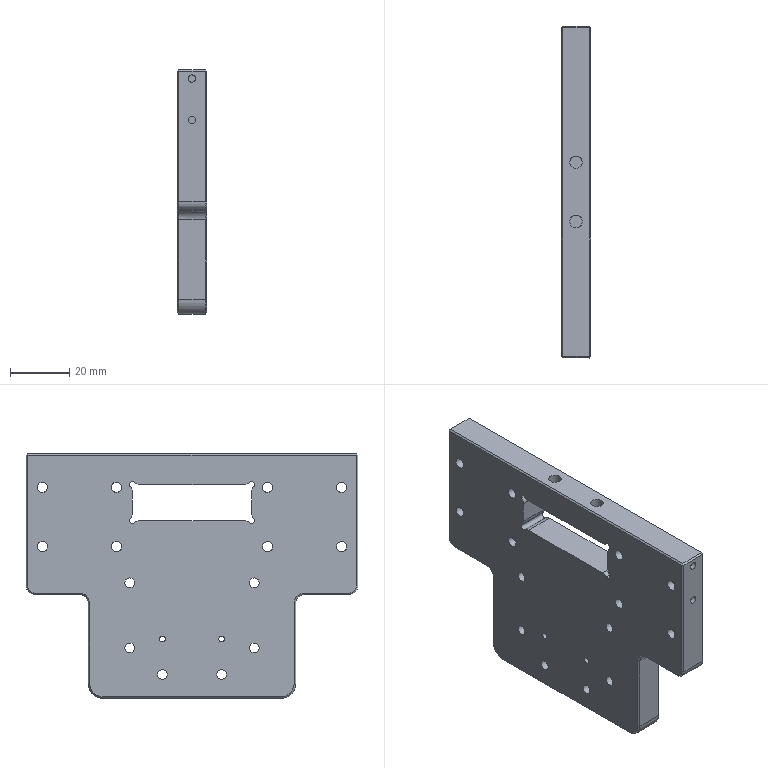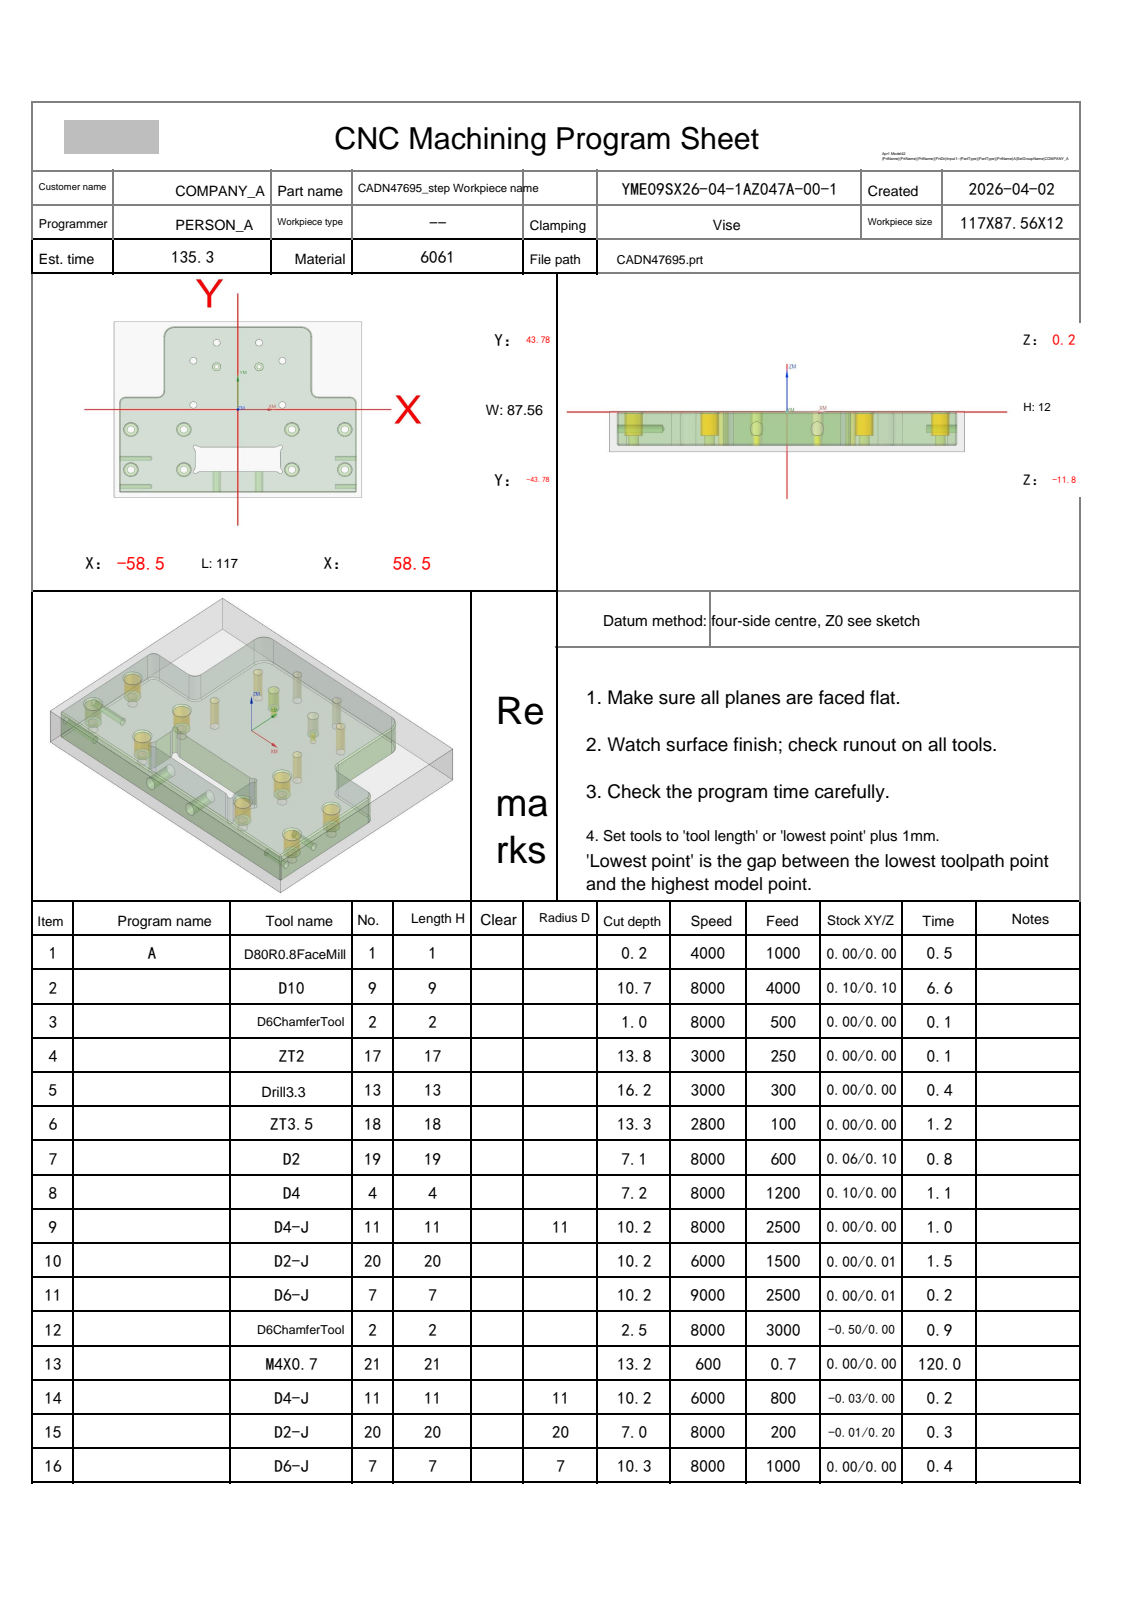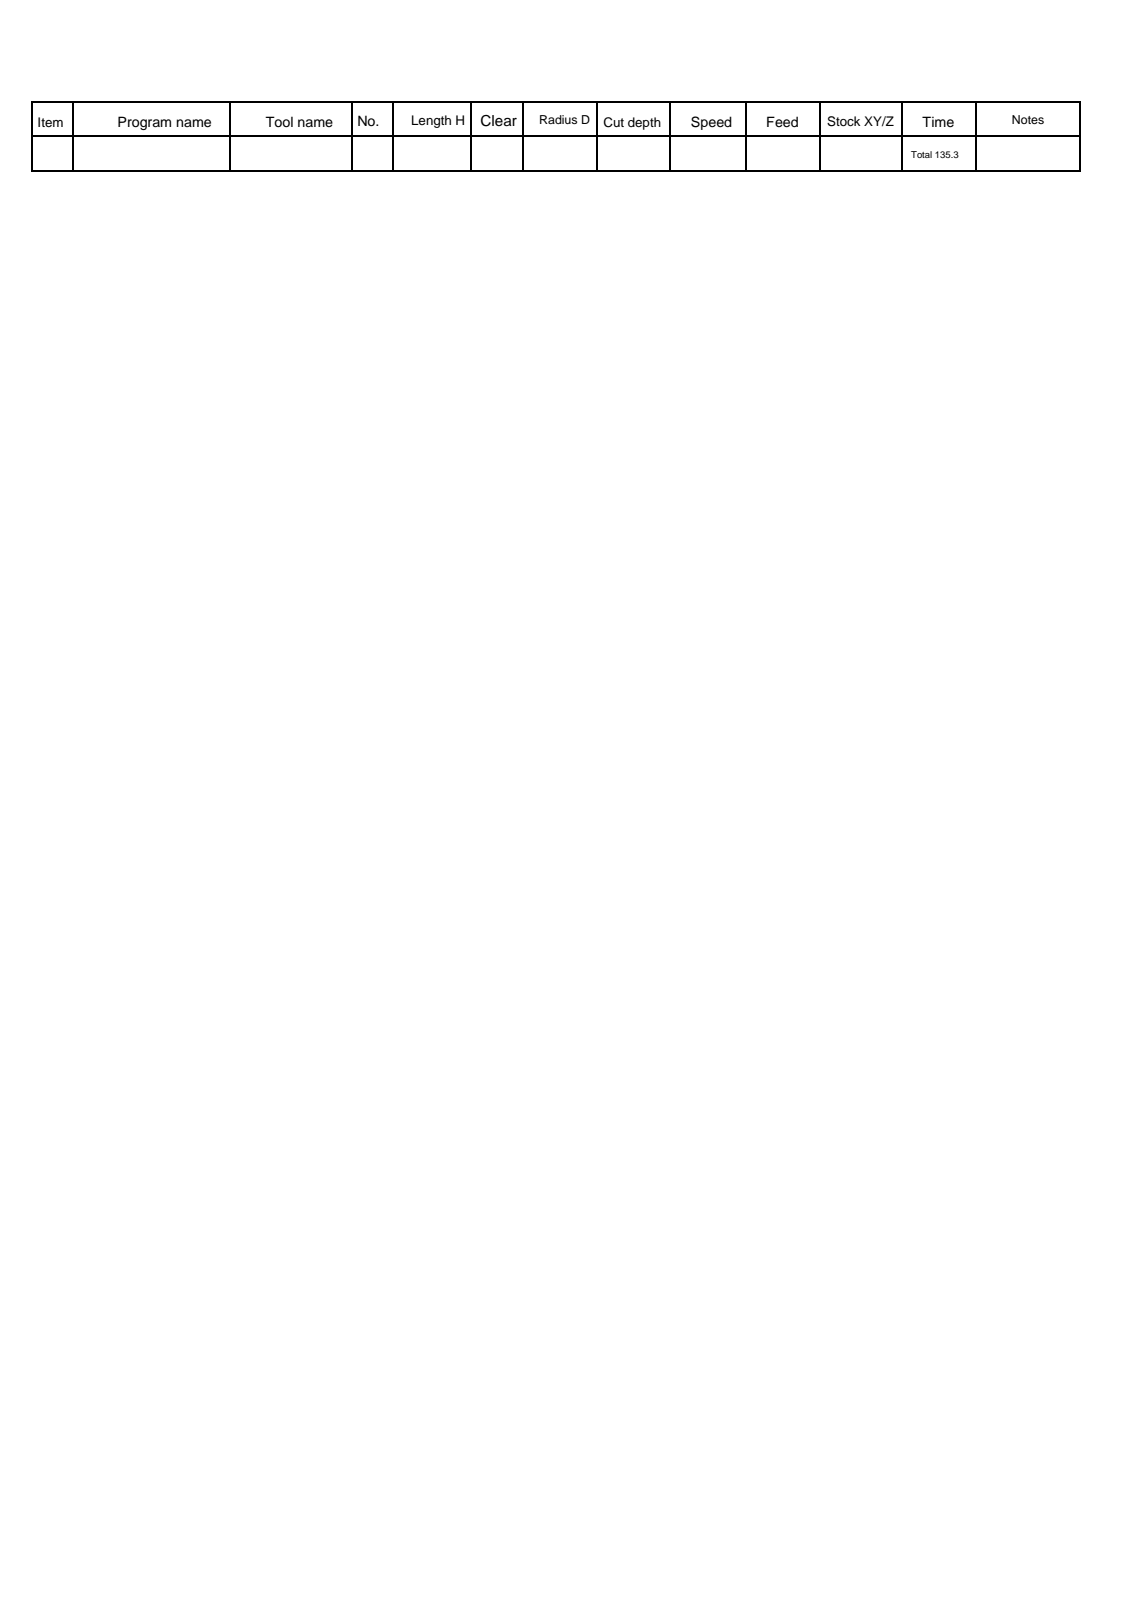NC program | NX | posted by the shop | part box 10 x 112 x 82.562 mm
Lines 1 to 40 of 16718:
%
O0001
(Machine time: 249.82 MIN)
(===Total Tool:12===)
(T1=D80R0.8 FaceMill D=80.  R=0.8  D-  H01 Z=-0.   )
(T9=D10     D=10.  R=0.   D-  H09 Z=-10.5 )
(T2=D6ChamferTool   D=6.   R=0.   D-  H02 Z=-2.3  )
(T17=ZT2    D=2.   DR_a=118 D-  H17 Z=-13.6 )
(T13=Drill 3.3  D=3.3  DR_a=118 D-  H13 Z=-15.99)
(T18=ZT3.5  D=3.5  DR_a=118 D-  H18 Z=-13.05)
(T19=D2     D=2.   R=0.   D-  H19 Z=-6.9  )
(T4=D4      D=4.   R=0.   D-  H04 Z=-7.   )
(T11=D4-J   D=4.   R=0.   D11 H11 Z=-10.  )
(T20=D2-J   D=2.   R=0.   D-  H20 Z=-10.  )
(T7=D6-J    D=6.   R=0.   D-  H07 Z=-10.1 )
(T21=M4X0.7 D=3.3  DR_a=180 D-  H21 Z=-13.  )
G80 G90 G17 G49 G40
G91 G28 Z0
M01
N1 T01 M06
(D80R0.8 FaceMill  D=80. R=0.8 H=01 ce=0.00 di=0.00)
G00 G90 G54 X101. Y-27.094 M03 S4000
G43 H01 Z20.
M08
Z2.
G01 Z0.0 F1000.
X96.
X-96.
Y27.094
X96.
X101.
Z2.
G00 Z20.
G91 G28 Z0.0
M05
M09
G91 G28 Z0.0
M01